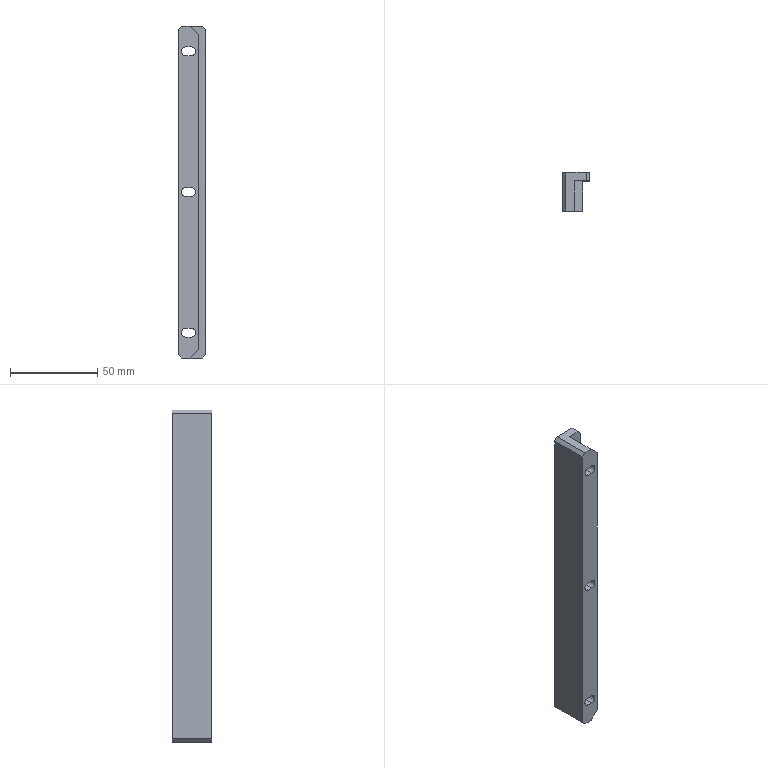Part | SolidWorks | features Chamfer 2, Extrusion 1, ICE 1 | 1 solid | 29 faces | box 16 x 22.5 x 190 mm | volume 52215 mm3 | plane 20 | cylinder 9 | commonest cylinder face diameters 5 x9
STEP:
#1=CARTESIAN_POINT('',(7.5,22.5,83.));
#2=VERTEX_POINT('',#1);
#3=CARTESIAN_POINT('',(10.,22.5,80.5));
#4=VERTEX_POINT('',#3);
#5=CARTESIAN_POINT('',(7.5,22.5,80.5));
#6=DIRECTION('',(0.,1.,0.));
#7=DIRECTION('',(0.,0.,-1.));
#8=AXIS2_PLACEMENT_3D('',#5,#6,#7);
#9=CIRCLE('',#8,2.5);
#10=EDGE_CURVE('',#2,#4,#9,.T.);
#11=ORIENTED_EDGE('',*,*,#10,.T.);
#12=CARTESIAN_POINT('',(10.,0.,80.5));
#13=VERTEX_POINT('',#12);
#14=CARTESIAN_POINT('',(10.,22.501,80.5));
#15=DIRECTION('',(0.,-1.,0.));
#16=VECTOR('',#15,1000.);
#17=LINE('',#14,#16);
#18=EDGE_CURVE('',#4,#13,#17,.T.);
#19=ORIENTED_EDGE('',*,*,#18,.T.);
#20=CARTESIAN_POINT('',(7.5,0.,83.));
#21=VERTEX_POINT('',#20);
#22=CARTESIAN_POINT('',(7.5,0.,80.5));
#23=DIRECTION('',(0.,-1.,0.));
#24=DIRECTION('',(1.,0.,0.));
#25=AXIS2_PLACEMENT_3D('',#22,#23,#24);
#26=CIRCLE('',#25,2.5);
#27=EDGE_CURVE('',#13,#21,#26,.T.);
#28=ORIENTED_EDGE('',*,*,#27,.T.);
#29=CARTESIAN_POINT('',(7.5,22.501,83.));
#30=DIRECTION('',(0.,-1.,0.));
#31=VECTOR('',#30,1000.);
#32=LINE('',#29,#31);
#33=EDGE_CURVE('',#2,#21,#32,.T.);
#34=ORIENTED_EDGE('',*,*,#33,.F.);
#35=EDGE_LOOP('',(#11,#19,#28,#34));
#36=FACE_OUTER_BOUND('',#35,.T.);
#37=CARTESIAN_POINT('',(7.5,22.501,80.5));
#38=DIRECTION('',(0.,-1.,0.));
#39=DIRECTION('',(1.,0.,0.));
#40=AXIS2_PLACEMENT_3D('',#37,#38,#39);
#41=CYLINDRICAL_SURFACE('',#40,2.5);
#42=ADVANCED_FACE('',(#36),#41,.F.);
#43=CARTESIAN_POINT('',(7.5,22.5,2.5));
#44=VERTEX_POINT('',#43);
#45=CARTESIAN_POINT('',(10.,22.5,0.));
#46=VERTEX_POINT('',#45);
#47=CARTESIAN_POINT('',(7.5,22.5,0.));
#48=DIRECTION('',(0.,1.,0.));
#49=DIRECTION('',(0.,0.,-1.));
#50=AXIS2_PLACEMENT_3D('',#47,#48,#49);
#51=CIRCLE('',#50,2.5);
#52=EDGE_CURVE('',#44,#46,#51,.T.);
#53=ORIENTED_EDGE('',*,*,#52,.T.);
#54=CARTESIAN_POINT('',(10.,0.,0.));
#55=VERTEX_POINT('',#54);
#56=CARTESIAN_POINT('',(10.,22.501,0.));
#57=DIRECTION('',(0.,-1.,0.));
#58=VECTOR('',#57,1000.);
#59=LINE('',#56,#58);
#60=EDGE_CURVE('',#46,#55,#59,.T.);
#61=ORIENTED_EDGE('',*,*,#60,.T.);
#62=CARTESIAN_POINT('',(7.5,0.,2.5));
#63=VERTEX_POINT('',#62);
#64=CARTESIAN_POINT('',(7.5,0.,0.));
#65=DIRECTION('',(0.,-1.,0.));
#66=DIRECTION('',(1.,0.,0.));
#67=AXIS2_PLACEMENT_3D('',#64,#65,#66);
#68=CIRCLE('',#67,2.5);
#69=EDGE_CURVE('',#55,#63,#68,.T.);
#70=ORIENTED_EDGE('',*,*,#69,.T.);
#71=CARTESIAN_POINT('',(7.5,22.501,2.5));
#72=DIRECTION('',(0.,-1.,0.));
#73=VECTOR('',#72,1000.);
#74=LINE('',#71,#73);
#75=EDGE_CURVE('',#44,#63,#74,.T.);
#76=ORIENTED_EDGE('',*,*,#75,.F.);
#77=EDGE_LOOP('',(#53,#61,#70,#76));
#78=FACE_OUTER_BOUND('',#77,.T.);
#79=CARTESIAN_POINT('',(7.5,22.501,0.));
#80=DIRECTION('',(0.,-1.,0.));
#81=DIRECTION('',(1.,0.,0.));
#82=AXIS2_PLACEMENT_3D('',#79,#80,#81);
#83=CYLINDRICAL_SURFACE('',#82,2.5);
#84=ADVANCED_FACE('',(#78),#83,.F.);
#85=CARTESIAN_POINT('',(7.5,22.5,-78.));
#86=VERTEX_POINT('',#85);
#87=CARTESIAN_POINT('',(10.,22.5,-80.5));
#88=VERTEX_POINT('',#87);
#89=CARTESIAN_POINT('',(7.5,22.5,-80.5));
#90=DIRECTION('',(0.,1.,0.));
#91=DIRECTION('',(0.,0.,-1.));
#92=AXIS2_PLACEMENT_3D('',#89,#90,#91);
#93=CIRCLE('',#92,2.5);
#94=EDGE_CURVE('',#86,#88,#93,.T.);
#95=ORIENTED_EDGE('',*,*,#94,.T.);
#96=CARTESIAN_POINT('',(10.,0.,-80.5));
#97=VERTEX_POINT('',#96);
#98=CARTESIAN_POINT('',(10.,22.501,-80.5));
#99=DIRECTION('',(0.,-1.,0.));
#100=VECTOR('',#99,1000.);
#101=LINE('',#98,#100);
#102=EDGE_CURVE('',#88,#97,#101,.T.);
#103=ORIENTED_EDGE('',*,*,#102,.T.);
#104=CARTESIAN_POINT('',(7.5,0.,-78.));
#105=VERTEX_POINT('',#104);
#106=CARTESIAN_POINT('',(7.5,0.,-80.5));
#107=DIRECTION('',(0.,-1.,0.));
#108=DIRECTION('',(-1.,0.,0.));
#109=AXIS2_PLACEMENT_3D('',#106,#107,#108);
#110=CIRCLE('',#109,2.5);
#111=EDGE_CURVE('',#97,#105,#110,.T.);
#112=ORIENTED_EDGE('',*,*,#111,.T.);
#113=CARTESIAN_POINT('',(7.5,22.501,-78.));
#114=DIRECTION('',(0.,-1.,0.));
#115=VECTOR('',#114,1000.);
#116=LINE('',#113,#115);
#117=EDGE_CURVE('',#86,#105,#116,.T.);
#118=ORIENTED_EDGE('',*,*,#117,.F.);
#119=EDGE_LOOP('',(#95,#103,#112,#118));
#120=FACE_OUTER_BOUND('',#119,.T.);
#121=CARTESIAN_POINT('',(7.5,22.501,-80.5));
#122=DIRECTION('',(0.,-1.,0.));
#123=DIRECTION('',(1.,0.,0.));
#124=AXIS2_PLACEMENT_3D('',#121,#122,#123);
#125=CYLINDRICAL_SURFACE('',#124,2.5);
#126=ADVANCED_FACE('',(#120),#125,.F.);
#127=CARTESIAN_POINT('',(4.5,0.,78.));
#128=VERTEX_POINT('',#127);
#129=CARTESIAN_POINT('',(7.5,0.,78.));
#130=VERTEX_POINT('',#129);
#131=CARTESIAN_POINT('',(4.5,0.,78.));
#132=DIRECTION('',(1.,0.,0.));
#133=VECTOR('',#132,1000.);
#134=LINE('',#131,#133);
#135=EDGE_CURVE('',#128,#130,#134,.T.);
#136=ORIENTED_EDGE('',*,*,#135,.F.);
#137=CARTESIAN_POINT('',(4.5,0.,83.));
#138=VERTEX_POINT('',#137);
#139=CARTESIAN_POINT('',(4.5,0.,80.5));
#140=DIRECTION('',(0.,-1.,0.));
#141=DIRECTION('',(1.,0.,0.));
#142=AXIS2_PLACEMENT_3D('',#139,#140,#141);
#143=CIRCLE('',#142,2.5);
#144=EDGE_CURVE('',#138,#128,#143,.T.);
#145=ORIENTED_EDGE('',*,*,#144,.F.);
#146=CARTESIAN_POINT('',(4.5,0.,83.));
#147=DIRECTION('',(-1.,0.,0.));
#148=VECTOR('',#147,1000.);
#149=LINE('',#146,#148);
#150=EDGE_CURVE('',#21,#138,#149,.T.);
#151=ORIENTED_EDGE('',*,*,#150,.F.);
#152=ORIENTED_EDGE('',*,*,#27,.F.);
#153=CARTESIAN_POINT('',(7.5,0.,80.5));
#154=DIRECTION('',(0.,-1.,0.));
#155=DIRECTION('',(1.,0.,0.));
#156=AXIS2_PLACEMENT_3D('',#153,#154,#155);
#157=CIRCLE('',#156,2.5);
#158=EDGE_CURVE('',#130,#13,#157,.T.);
#159=ORIENTED_EDGE('',*,*,#158,.F.);
#160=EDGE_LOOP('',(#136,#145,#151,#152,#159));
#161=FACE_BOUND('',#160,.T.);
#162=CARTESIAN_POINT('',(4.5,0.,-2.5));
#163=VERTEX_POINT('',#162);
#164=CARTESIAN_POINT('',(7.5,0.,-2.5));
#165=VERTEX_POINT('',#164);
#166=CARTESIAN_POINT('',(4.5,0.,-2.5));
#167=DIRECTION('',(1.,0.,0.));
#168=VECTOR('',#167,1000.);
#169=LINE('',#166,#168);
#170=EDGE_CURVE('',#163,#165,#169,.T.);
#171=ORIENTED_EDGE('',*,*,#170,.F.);
#172=CARTESIAN_POINT('',(4.5,0.,2.5));
#173=VERTEX_POINT('',#172);
#174=CARTESIAN_POINT('',(4.5,0.,0.));
#175=DIRECTION('',(0.,-1.,0.));
#176=DIRECTION('',(1.,0.,0.));
#177=AXIS2_PLACEMENT_3D('',#174,#175,#176);
#178=CIRCLE('',#177,2.5);
#179=EDGE_CURVE('',#173,#163,#178,.T.);
#180=ORIENTED_EDGE('',*,*,#179,.F.);
#181=CARTESIAN_POINT('',(4.5,0.,2.5));
#182=DIRECTION('',(-1.,0.,0.));
#183=VECTOR('',#182,1000.);
#184=LINE('',#181,#183);
#185=EDGE_CURVE('',#63,#173,#184,.T.);
#186=ORIENTED_EDGE('',*,*,#185,.F.);
#187=ORIENTED_EDGE('',*,*,#69,.F.);
#188=CARTESIAN_POINT('',(7.5,0.,0.));
#189=DIRECTION('',(0.,-1.,0.));
#190=DIRECTION('',(1.,0.,0.));
#191=AXIS2_PLACEMENT_3D('',#188,#189,#190);
#192=CIRCLE('',#191,2.5);
#193=EDGE_CURVE('',#165,#55,#192,.T.);
#194=ORIENTED_EDGE('',*,*,#193,.F.);
#195=EDGE_LOOP('',(#171,#180,#186,#187,#194));
#196=FACE_BOUND('',#195,.T.);
#197=CARTESIAN_POINT('',(4.5,0.,-83.));
#198=VERTEX_POINT('',#197);
#199=CARTESIAN_POINT('',(7.5,0.,-83.));
#200=VERTEX_POINT('',#199);
#201=CARTESIAN_POINT('',(4.5,0.,-83.));
#202=DIRECTION('',(1.,0.,0.));
#203=VECTOR('',#202,1000.);
#204=LINE('',#201,#203);
#205=EDGE_CURVE('',#198,#200,#204,.T.);
#206=ORIENTED_EDGE('',*,*,#205,.F.);
#207=CARTESIAN_POINT('',(4.5,0.,-78.));
#208=VERTEX_POINT('',#207);
#209=CARTESIAN_POINT('',(4.5,0.,-80.5));
#210=DIRECTION('',(0.,-1.,0.));
#211=DIRECTION('',(-1.,0.,0.));
#212=AXIS2_PLACEMENT_3D('',#209,#210,#211);
#213=CIRCLE('',#212,2.5);
#214=EDGE_CURVE('',#208,#198,#213,.T.);
#215=ORIENTED_EDGE('',*,*,#214,.F.);
#216=CARTESIAN_POINT('',(4.5,0.,-78.));
#217=DIRECTION('',(-1.,0.,0.));
#218=VECTOR('',#217,1000.);
#219=LINE('',#216,#218);
#220=EDGE_CURVE('',#105,#208,#219,.T.);
#221=ORIENTED_EDGE('',*,*,#220,.F.);
#222=ORIENTED_EDGE('',*,*,#111,.F.);
#223=CARTESIAN_POINT('',(7.5,0.,-80.5));
#224=DIRECTION('',(0.,-1.,0.));
#225=DIRECTION('',(-1.,0.,0.));
#226=AXIS2_PLACEMENT_3D('',#223,#224,#225);
#227=CIRCLE('',#226,2.5);
#228=EDGE_CURVE('',#200,#97,#227,.T.);
#229=ORIENTED_EDGE('',*,*,#228,.F.);
#230=EDGE_LOOP('',(#206,#215,#221,#222,#229));
#231=FACE_BOUND('',#230,.T.);
#232=CARTESIAN_POINT('',(2.,0.,95.));
#233=VERTEX_POINT('',#232);
#234=CARTESIAN_POINT('',(7.,0.,95.));
#235=VERTEX_POINT('',#234);
#236=CARTESIAN_POINT('',(12.,0.,95.));
#237=DIRECTION('',(1.,0.,0.));
#238=VECTOR('',#237,1000.);
#239=LINE('',#236,#238);
#240=EDGE_CURVE('',#233,#235,#239,.T.);
#241=ORIENTED_EDGE('',*,*,#240,.F.);
#242=CARTESIAN_POINT('',(0.,0.,93.));
#243=VERTEX_POINT('',#242);
#244=CARTESIAN_POINT('',(2.,0.,95.));
#245=DIRECTION('',(-0.7071,0.,-0.7071));
#246=VECTOR('',#245,1000.);
#247=LINE('',#244,#246);
#248=EDGE_CURVE('',#233,#243,#247,.T.);
#249=ORIENTED_EDGE('',*,*,#248,.T.);
#250=CARTESIAN_POINT('',(0.,0.,-93.));
#251=VERTEX_POINT('',#250);
#252=CARTESIAN_POINT('',(0.,0.,95.));
#253=DIRECTION('',(0.,0.,-1.));
#254=VECTOR('',#253,1000.);
#255=LINE('',#252,#254);
#256=EDGE_CURVE('',#243,#251,#255,.T.);
#257=ORIENTED_EDGE('',*,*,#256,.T.);
#258=CARTESIAN_POINT('',(2.,0.,-95.));
#259=VERTEX_POINT('',#258);
#260=CARTESIAN_POINT('',(0.,0.,-93.));
#261=DIRECTION('',(0.7071,0.,-0.7071));
#262=VECTOR('',#261,1000.);
#263=LINE('',#260,#262);
#264=EDGE_CURVE('',#251,#259,#263,.T.);
#265=ORIENTED_EDGE('',*,*,#264,.T.);
#266=CARTESIAN_POINT('',(7.,0.,-95.));
#267=VERTEX_POINT('',#266);
#268=CARTESIAN_POINT('',(12.,0.,-95.));
#269=DIRECTION('',(1.,0.,0.));
#270=VECTOR('',#269,1000.);
#271=LINE('',#268,#270);
#272=EDGE_CURVE('',#259,#267,#271,.T.);
#273=ORIENTED_EDGE('',*,*,#272,.T.);
#274=CARTESIAN_POINT('',(12.,0.,-90.));
#275=VERTEX_POINT('',#274);
#276=CARTESIAN_POINT('',(12.,0.,-90.));
#277=DIRECTION('',(0.7071,0.,0.7071));
#278=VECTOR('',#277,1000.);
#279=LINE('',#276,#278);
#280=EDGE_CURVE('',#267,#275,#279,.T.);
#281=ORIENTED_EDGE('',*,*,#280,.T.);
#282=CARTESIAN_POINT('',(12.,0.,90.));
#283=VERTEX_POINT('',#282);
#284=CARTESIAN_POINT('',(12.,0.,95.));
#285=DIRECTION('',(0.,0.,-1.));
#286=VECTOR('',#285,1000.);
#287=LINE('',#284,#286);
#288=EDGE_CURVE('',#283,#275,#287,.T.);
#289=ORIENTED_EDGE('',*,*,#288,.F.);
#290=CARTESIAN_POINT('',(7.,0.,95.));
#291=DIRECTION('',(-0.7071,0.,0.7071));
#292=VECTOR('',#291,1000.);
#293=LINE('',#290,#292);
#294=EDGE_CURVE('',#283,#235,#293,.T.);
#295=ORIENTED_EDGE('',*,*,#294,.T.);
#296=EDGE_LOOP('',(#241,#249,#257,#265,#273,#281,#289,#295));
#297=FACE_OUTER_BOUND('',#296,.T.);
#298=CARTESIAN_POINT('',(12.,0.,95.));
#299=DIRECTION('',(0.,1.,0.));
#300=DIRECTION('',(-1.,0.,0.));
#301=AXIS2_PLACEMENT_3D('',#298,#299,#300);
#302=PLANE('',#301);
#303=ADVANCED_FACE('',(#161,#196,#231,#297),#302,.F.);
#304=ORIENTED_EDGE('',*,*,#288,.T.);
#305=CARTESIAN_POINT('',(12.,17.5,-90.));
#306=VERTEX_POINT('',#305);
#307=CARTESIAN_POINT('',(12.,17.5,-90.));
#308=DIRECTION('',(0.,1.,0.));
#309=VECTOR('',#308,1000.);
#310=LINE('',#307,#309);
#311=EDGE_CURVE('',#275,#306,#310,.T.);
#312=ORIENTED_EDGE('',*,*,#311,.T.);
#313=CARTESIAN_POINT('',(12.,17.5,90.));
#314=VERTEX_POINT('',#313);
#315=CARTESIAN_POINT('',(12.,17.5,95.));
#316=DIRECTION('',(0.,0.,-1.));
#317=VECTOR('',#316,1000.);
#318=LINE('',#315,#317);
#319=EDGE_CURVE('',#314,#306,#318,.T.);
#320=ORIENTED_EDGE('',*,*,#319,.F.);
#321=CARTESIAN_POINT('',(12.,17.5,90.));
#322=DIRECTION('',(0.,-1.,0.));
#323=VECTOR('',#322,1000.);
#324=LINE('',#321,#323);
#325=EDGE_CURVE('',#314,#283,#324,.T.);
#326=ORIENTED_EDGE('',*,*,#325,.T.);
#327=EDGE_LOOP('',(#304,#312,#320,#326));
#328=FACE_OUTER_BOUND('',#327,.T.);
#329=CARTESIAN_POINT('',(12.,17.5,95.));
#330=DIRECTION('',(-1.,0.,0.));
#331=DIRECTION('',(0.,-1.,0.));
#332=AXIS2_PLACEMENT_3D('',#329,#330,#331);
#333=PLANE('',#332);
#334=ADVANCED_FACE('',(#328),#333,.F.);
#335=CARTESIAN_POINT('',(7.,17.5,-95.));
#336=VERTEX_POINT('',#335);
#337=CARTESIAN_POINT('',(14.,17.5,-95.));
#338=VERTEX_POINT('',#337);
#339=CARTESIAN_POINT('',(16.,17.5,-95.));
#340=DIRECTION('',(1.,0.,0.));
#341=VECTOR('',#340,1000.);
#342=LINE('',#339,#341);
#343=EDGE_CURVE('',#336,#338,#342,.T.);
#344=ORIENTED_EDGE('',*,*,#343,.T.);
#345=CARTESIAN_POINT('',(16.,17.5,-93.));
#346=VERTEX_POINT('',#345);
#347=CARTESIAN_POINT('',(16.,17.5,-93.));
#348=DIRECTION('',(0.7071,0.,0.7071));
#349=VECTOR('',#348,1000.);
#350=LINE('',#347,#349);
#351=EDGE_CURVE('',#338,#346,#350,.T.);
#352=ORIENTED_EDGE('',*,*,#351,.T.);
#353=CARTESIAN_POINT('',(16.,17.5,93.));
#354=VERTEX_POINT('',#353);
#355=CARTESIAN_POINT('',(16.,17.5,95.));
#356=DIRECTION('',(0.,0.,-1.));
#357=VECTOR('',#356,1000.);
#358=LINE('',#355,#357);
#359=EDGE_CURVE('',#354,#346,#358,.T.);
#360=ORIENTED_EDGE('',*,*,#359,.F.);
#361=CARTESIAN_POINT('',(14.,17.5,95.));
#362=VERTEX_POINT('',#361);
#363=CARTESIAN_POINT('',(14.,17.5,95.));
#364=DIRECTION('',(-0.7071,0.,0.7071));
#365=VECTOR('',#364,1000.);
#366=LINE('',#363,#365);
#367=EDGE_CURVE('',#354,#362,#366,.T.);
#368=ORIENTED_EDGE('',*,*,#367,.T.);
#369=CARTESIAN_POINT('',(7.,17.5,95.));
#370=VERTEX_POINT('',#369);
#371=CARTESIAN_POINT('',(16.,17.5,95.));
#372=DIRECTION('',(1.,0.,0.));
#373=VECTOR('',#372,1000.);
#374=LINE('',#371,#373);
#375=EDGE_CURVE('',#370,#362,#374,.T.);
#376=ORIENTED_EDGE('',*,*,#375,.F.);
#377=CARTESIAN_POINT('',(11.5,17.5,90.5));
#378=DIRECTION('',(0.7071,0.,-0.7071));
#379=VECTOR('',#378,1000.);
#380=LINE('',#377,#379);
#381=EDGE_CURVE('',#370,#314,#380,.T.);
#382=ORIENTED_EDGE('',*,*,#381,.T.);
#383=ORIENTED_EDGE('',*,*,#319,.T.);
#384=CARTESIAN_POINT('',(106.5,17.5,4.5));
#385=DIRECTION('',(-0.7071,0.,-0.7071));
#386=VECTOR('',#385,1000.);
#387=LINE('',#384,#386);
#388=EDGE_CURVE('',#306,#336,#387,.T.);
#389=ORIENTED_EDGE('',*,*,#388,.T.);
#390=EDGE_LOOP('',(#344,#352,#360,#368,#376,#382,#383,#389));
#391=FACE_OUTER_BOUND('',#390,.T.);
#392=CARTESIAN_POINT('',(16.,17.5,95.));
#393=DIRECTION('',(0.,1.,0.));
#394=DIRECTION('',(0.,0.,1.));
#395=AXIS2_PLACEMENT_3D('',#392,#393,#394);
#396=PLANE('',#395);
#397=ADVANCED_FACE('',(#391),#396,.F.);
#398=ORIENTED_EDGE('',*,*,#359,.T.);
#399=CARTESIAN_POINT('',(16.,22.5,-93.));
#400=VERTEX_POINT('',#399);
#401=CARTESIAN_POINT('',(16.,22.5,-93.));
#402=DIRECTION('',(0.,1.,0.));
#403=VECTOR('',#402,1000.);
#404=LINE('',#401,#403);
#405=EDGE_CURVE('',#346,#400,#404,.T.);
#406=ORIENTED_EDGE('',*,*,#405,.T.);
#407=CARTESIAN_POINT('',(16.,22.5,93.));
#408=VERTEX_POINT('',#407);
#409=CARTESIAN_POINT('',(16.,22.5,95.));
#410=DIRECTION('',(0.,0.,-1.));
#411=VECTOR('',#410,1000.);
#412=LINE('',#409,#411);
#413=EDGE_CURVE('',#408,#400,#412,.T.);
#414=ORIENTED_EDGE('',*,*,#413,.F.);
#415=CARTESIAN_POINT('',(16.,22.5,93.));
#416=DIRECTION('',(0.,-1.,0.));
#417=VECTOR('',#416,1000.);
#418=LINE('',#415,#417);
#419=EDGE_CURVE('',#408,#354,#418,.T.);
#420=ORIENTED_EDGE('',*,*,#419,.T.);
#421=EDGE_LOOP('',(#398,#406,#414,#420));
#422=FACE_OUTER_BOUND('',#421,.T.);
#423=CARTESIAN_POINT('',(16.,22.5,95.));
#424=DIRECTION('',(-1.,0.,0.));
#425=DIRECTION('',(0.,0.,1.));
#426=AXIS2_PLACEMENT_3D('',#423,#424,#425);
#427=PLANE('',#426);
#428=ADVANCED_FACE('',(#422),#427,.F.);
#429=CARTESIAN_POINT('',(4.5,22.5,83.));
#430=VERTEX_POINT('',#429);
#431=CARTESIAN_POINT('',(4.5,22.5,83.));
#432=DIRECTION('',(1.,0.,0.));
#433=VECTOR('',#432,1000.);
#434=LINE('',#431,#433);
#435=EDGE_CURVE('',#430,#2,#434,.T.);
#436=ORIENTED_EDGE('',*,*,#435,.F.);
#437=CARTESIAN_POINT('',(4.5,22.5,78.));
#438=VERTEX_POINT('',#437);
#439=CARTESIAN_POINT('',(4.5,22.5,80.5));
#440=DIRECTION('',(0.,1.,0.));
#441=DIRECTION('',(0.,0.,-1.));
#442=AXIS2_PLACEMENT_3D('',#439,#440,#441);
#443=CIRCLE('',#442,2.5);
#444=EDGE_CURVE('',#438,#430,#443,.T.);
#445=ORIENTED_EDGE('',*,*,#444,.F.);
#446=CARTESIAN_POINT('',(7.5,22.5,78.));
#447=VERTEX_POINT('',#446);
#448=CARTESIAN_POINT('',(4.5,22.5,78.));
#449=DIRECTION('',(-1.,0.,0.));
#450=VECTOR('',#449,1000.);
#451=LINE('',#448,#450);
#452=EDGE_CURVE('',#447,#438,#451,.T.);
#453=ORIENTED_EDGE('',*,*,#452,.F.);
#454=CARTESIAN_POINT('',(7.5,22.5,80.5));
#455=DIRECTION('',(0.,1.,0.));
#456=DIRECTION('',(0.,0.,-1.));
#457=AXIS2_PLACEMENT_3D('',#454,#455,#456);
#458=CIRCLE('',#457,2.5);
#459=EDGE_CURVE('',#4,#447,#458,.T.);
#460=ORIENTED_EDGE('',*,*,#459,.F.);
#461=ORIENTED_EDGE('',*,*,#10,.F.);
#462=EDGE_LOOP('',(#436,#445,#453,#460,#461));
#463=FACE_BOUND('',#462,.T.);
#464=CARTESIAN_POINT('',(4.5,22.5,2.5));
#465=VERTEX_POINT('',#464);
#466=CARTESIAN_POINT('',(4.5,22.5,2.5));
#467=DIRECTION('',(1.,0.,0.));
#468=VECTOR('',#467,1000.);
#469=LINE('',#466,#468);
#470=EDGE_CURVE('',#465,#44,#469,.T.);
#471=ORIENTED_EDGE('',*,*,#470,.F.);
#472=CARTESIAN_POINT('',(4.5,22.5,-2.5));
#473=VERTEX_POINT('',#472);
#474=CARTESIAN_POINT('',(4.5,22.5,0.));
#475=DIRECTION('',(0.,1.,0.));
#476=DIRECTION('',(0.,0.,-1.));
#477=AXIS2_PLACEMENT_3D('',#474,#475,#476);
#478=CIRCLE('',#477,2.5);
#479=EDGE_CURVE('',#473,#465,#478,.T.);
#480=ORIENTED_EDGE('',*,*,#479,.F.);
#481=CARTESIAN_POINT('',(7.5,22.5,-2.5));
#482=VERTEX_POINT('',#481);
#483=CARTESIAN_POINT('',(4.5,22.5,-2.5));
#484=DIRECTION('',(-1.,0.,0.));
#485=VECTOR('',#484,1000.);
#486=LINE('',#483,#485);
#487=EDGE_CURVE('',#482,#473,#486,.T.);
#488=ORIENTED_EDGE('',*,*,#487,.F.);
#489=CARTESIAN_POINT('',(7.5,22.5,0.));
#490=DIRECTION('',(0.,1.,0.));
#491=DIRECTION('',(0.,0.,-1.));
#492=AXIS2_PLACEMENT_3D('',#489,#490,#491);
#493=CIRCLE('',#492,2.5);
#494=EDGE_CURVE('',#46,#482,#493,.T.);
#495=ORIENTED_EDGE('',*,*,#494,.F.);
#496=ORIENTED_EDGE('',*,*,#52,.F.);
#497=EDGE_LOOP('',(#471,#480,#488,#495,#496));
#498=FACE_BOUND('',#497,.T.);
#499=CARTESIAN_POINT('',(4.5,22.5,-78.));
#500=VERTEX_POINT('',#499);
#501=CARTESIAN_POINT('',(4.5,22.5,-78.));
#502=DIRECTION('',(1.,0.,0.));
#503=VECTOR('',#502,1000.);
#504=LINE('',#501,#503);
#505=EDGE_CURVE('',#500,#86,#504,.T.);
#506=ORIENTED_EDGE('',*,*,#505,.F.);
#507=CARTESIAN_POINT('',(4.5,22.5,-83.));
#508=VERTEX_POINT('',#507);
#509=CARTESIAN_POINT('',(4.5,22.5,-80.5));
#510=DIRECTION('',(0.,1.,0.));
#511=DIRECTION('',(0.,0.,-1.));
#512=AXIS2_PLACEMENT_3D('',#509,#510,#511);
#513=CIRCLE('',#512,2.5);
#514=EDGE_CURVE('',#508,#500,#513,.T.);
#515=ORIENTED_EDGE('',*,*,#514,.F.);
#516=CARTESIAN_POINT('',(7.5,22.5,-83.));
#517=VERTEX_POINT('',#516);
#518=CARTESIAN_POINT('',(4.5,22.5,-83.));
#519=DIRECTION('',(-1.,0.,0.));
#520=VECTOR('',#519,1000.);
#521=LINE('',#518,#520);
#522=EDGE_CURVE('',#517,#508,#521,.T.);
#523=ORIENTED_EDGE('',*,*,#522,.F.);
#524=CARTESIAN_POINT('',(7.5,22.5,-80.5));
#525=DIRECTION('',(0.,1.,0.));
#526=DIRECTION('',(0.,0.,-1.));
#527=AXIS2_PLACEMENT_3D('',#524,#525,#526);
#528=CIRCLE('',#527,2.5);
#529=EDGE_CURVE('',#88,#517,#528,.T.);
#530=ORIENTED_EDGE('',*,*,#529,.F.);
#531=ORIENTED_EDGE('',*,*,#94,.F.);
#532=EDGE_LOOP('',(#506,#515,#523,#530,#531));
#533=FACE_BOUND('',#532,.T.);
#534=CARTESIAN_POINT('',(0.,22.5,93.));
#535=VERTEX_POINT('',#534);
#536=CARTESIAN_POINT('',(0.,22.5,-93.));
#537=VERTEX_POINT('',#536);
#538=CARTESIAN_POINT('',(0.,22.5,95.));
#539=DIRECTION('',(0.,0.,-1.));
#540=VECTOR('',#539,1000.);
#541=LINE('',#538,#540);
#542=EDGE_CURVE('',#535,#537,#541,.T.);
#543=ORIENTED_EDGE('',*,*,#542,.F.);
#544=CARTESIAN_POINT('',(2.,22.5,95.));
#545=VERTEX_POINT('',#544);
#546=CARTESIAN_POINT('',(2.,22.5,95.));
#547=DIRECTION('',(0.7071,0.,0.7071));
#548=VECTOR('',#547,1000.);
#549=LINE('',#546,#548);
#550=EDGE_CURVE('',#535,#545,#549,.T.);
#551=ORIENTED_EDGE('',*,*,#550,.T.);
#552=CARTESIAN_POINT('',(14.,22.5,95.));
#553=VERTEX_POINT('',#552);
#554=CARTESIAN_POINT('',(0.,22.5,95.));
#555=DIRECTION('',(-1.,0.,0.));
#556=VECTOR('',#555,1000.);
#557=LINE('',#554,#556);
#558=EDGE_CURVE('',#553,#545,#557,.T.);
#559=ORIENTED_EDGE('',*,*,#558,.F.);
#560=CARTESIAN_POINT('',(14.,22.5,95.));
#561=DIRECTION('',(0.7071,0.,-0.7071));
#562=VECTOR('',#561,1000.);
#563=LINE('',#560,#562);
#564=EDGE_CURVE('',#553,#408,#563,.T.);
#565=ORIENTED_EDGE('',*,*,#564,.T.);
#566=ORIENTED_EDGE('',*,*,#413,.T.);
#567=CARTESIAN_POINT('',(14.,22.5,-95.));
#568=VERTEX_POINT('',#567);
#569=CARTESIAN_POINT('',(16.,22.5,-93.));
#570=DIRECTION('',(-0.7071,0.,-0.7071));
#571=VECTOR('',#570,1000.);
#572=LINE('',#569,#571);
#573=EDGE_CURVE('',#400,#568,#572,.T.);
#574=ORIENTED_EDGE('',*,*,#573,.T.);
#575=CARTESIAN_POINT('',(2.,22.5,-95.));
#576=VERTEX_POINT('',#575);
#577=CARTESIAN_POINT('',(0.,22.5,-95.));
#578=DIRECTION('',(-1.,0.,0.));
#579=VECTOR('',#578,1000.);
#580=LINE('',#577,#579);
#581=EDGE_CURVE('',#568,#576,#580,.T.);
#582=ORIENTED_EDGE('',*,*,#581,.T.);
#583=CARTESIAN_POINT('',(0.,22.5,-93.));
#584=DIRECTION('',(-0.7071,0.,0.7071));
#585=VECTOR('',#584,1000.);
#586=LINE('',#583,#585);
#587=EDGE_CURVE('',#576,#537,#586,.T.);
#588=ORIENTED_EDGE('',*,*,#587,.T.);
#589=EDGE_LOOP('',(#543,#551,#559,#565,#566,#574,#582,#588));
#590=FACE_OUTER_BOUND('',#589,.T.);
#591=CARTESIAN_POINT('',(0.,22.5,95.));
#592=DIRECTION('',(0.,-1.,0.));
#593=DIRECTION('',(0.,0.,-1.));
#594=AXIS2_PLACEMENT_3D('',#591,#592,#593);
#595=PLANE('',#594);
#596=ADVANCED_FACE('',(#463,#498,#533,#590),#595,.F.);
#597=ORIENTED_EDGE('',*,*,#256,.F.);
#598=CARTESIAN_POINT('',(0.,0.,93.));
#599=DIRECTION('',(0.,1.,0.));
#600=VECTOR('',#599,1000.);
#601=LINE('',#598,#600);
#602=EDGE_CURVE('',#243,#535,#601,.T.);
#603=ORIENTED_EDGE('',*,*,#602,.T.);
#604=ORIENTED_EDGE('',*,*,#542,.T.);
#605=CARTESIAN_POINT('',(0.,0.,-93.));
#606=DIRECTION('',(0.,-1.,0.));
#607=VECTOR('',#606,1000.);
#608=LINE('',#605,#607);
#609=EDGE_CURVE('',#537,#251,#608,.T.);
#610=ORIENTED_EDGE('',*,*,#609,.T.);
#611=EDGE_LOOP('',(#597,#603,#604,#610));
#612=FACE_OUTER_BOUND('',#611,.T.);
#613=CARTESIAN_POINT('',(0.,0.,95.));
#614=DIRECTION('',(1.,0.,0.));
#615=DIRECTION('',(0.,0.,-1.));
#616=AXIS2_PLACEMENT_3D('',#613,#614,#615);
#617=PLANE('',#616);
#618=ADVANCED_FACE('',(#612),#617,.F.);
#619=ORIENTED_EDGE('',*,*,#558,.T.);
#620=CARTESIAN_POINT('',(2.,0.,95.));
#621=DIRECTION('',(0.,-1.,0.));
#622=VECTOR('',#621,1000.);
#623=LINE('',#620,#622);
#624=EDGE_CURVE('',#545,#233,#623,.T.);
#625=ORIENTED_EDGE('',*,*,#624,.T.);
#626=ORIENTED_EDGE('',*,*,#240,.T.);
#627=CARTESIAN_POINT('',(7.,0.,95.));
#628=DIRECTION('',(0.,1.,0.));
#629=VECTOR('',#628,1000.);
#630=LINE('',#627,#629);
#631=EDGE_CURVE('',#235,#370,#630,.T.);
#632=ORIENTED_EDGE('',*,*,#631,.T.);
#633=ORIENTED_EDGE('',*,*,#375,.T.);
#634=CARTESIAN_POINT('',(14.,0.,95.));
#635=DIRECTION('',(0.,1.,0.));
#636=VECTOR('',#635,1000.);
#637=LINE('',#634,#636);
#638=EDGE_CURVE('',#362,#553,#637,.T.);
#639=ORIENTED_EDGE('',*,*,#638,.T.);
#640=EDGE_LOOP('',(#619,#625,#626,#632,#633,#639));
#641=FACE_OUTER_BOUND('',#640,.T.);
#642=CARTESIAN_POINT('',(0.,0.,95.));
#643=DIRECTION('',(0.,0.,-1.));
#644=DIRECTION('',(-1.,0.,0.));
#645=AXIS2_PLACEMENT_3D('',#642,#643,#644);
#646=PLANE('',#645);
#647=ADVANCED_FACE('',(#641),#646,.F.);
#648=ORIENTED_EDGE('',*,*,#272,.F.);
#649=CARTESIAN_POINT('',(2.,22.5,-95.));
#650=DIRECTION('',(0.,1.,0.));
#651=VECTOR('',#650,1000.);
#652=LINE('',#649,#651);
#653=EDGE_CURVE('',#259,#576,#652,.T.);
#654=ORIENTED_EDGE('',*,*,#653,.T.);
#655=ORIENTED_EDGE('',*,*,#581,.F.);
#656=CARTESIAN_POINT('',(14.,17.5,-95.));
#657=DIRECTION('',(0.,-1.,0.));
#658=VECTOR('',#657,1000.);
#659=LINE('',#656,#658);
#660=EDGE_CURVE('',#568,#338,#659,.T.);
#661=ORIENTED_EDGE('',*,*,#660,.T.);
#662=ORIENTED_EDGE('',*,*,#343,.F.);
#663=CARTESIAN_POINT('',(7.,0.,-95.));
#664=DIRECTION('',(0.,-1.,0.));
#665=VECTOR('',#664,1000.);
#666=LINE('',#663,#665);
#667=EDGE_CURVE('',#336,#267,#666,.T.);
#668=ORIENTED_EDGE('',*,*,#667,.T.);
#669=EDGE_LOOP('',(#648,#654,#655,#661,#662,#668));
#670=FACE_OUTER_BOUND('',#669,.T.);
#671=CARTESIAN_POINT('',(0.,0.,-95.));
#672=DIRECTION('',(0.,0.,-1.));
#673=DIRECTION('',(-1.,0.,0.));
#674=AXIS2_PLACEMENT_3D('',#671,#672,#673);
#675=PLANE('',#674);
#676=ADVANCED_FACE('',(#670),#675,.T.);
#677=ORIENTED_EDGE('',*,*,#280,.F.);
#678=ORIENTED_EDGE('',*,*,#667,.F.);
#679=ORIENTED_EDGE('',*,*,#388,.F.);
#680=ORIENTED_EDGE('',*,*,#311,.F.);
#681=EDGE_LOOP('',(#677,#678,#679,#680));
#682=FACE_OUTER_BOUND('',#681,.T.);
#683=CARTESIAN_POINT('',(12.,17.5,-90.));
#684=DIRECTION('',(0.7071,0.,-0.7071));
#685=DIRECTION('',(0.,-1.,0.));
#686=AXIS2_PLACEMENT_3D('',#683,#684,#685);
#687=PLANE('',#686);
#688=ADVANCED_FACE('',(#682),#687,.T.);
#689=ORIENTED_EDGE('',*,*,#294,.F.);
#690=ORIENTED_EDGE('',*,*,#325,.F.);
#691=ORIENTED_EDGE('',*,*,#381,.F.);
#692=ORIENTED_EDGE('',*,*,#631,.F.);
#693=EDGE_LOOP('',(#689,#690,#691,#692));
#694=FACE_OUTER_BOUND('',#693,.T.);
#695=CARTESIAN_POINT('',(7.,0.,95.));
#696=DIRECTION('',(-0.7071,0.,-0.7071));
#697=DIRECTION('',(0.,1.,0.));
#698=AXIS2_PLACEMENT_3D('',#695,#696,#697);
#699=PLANE('',#698);
#700=ADVANCED_FACE('',(#694),#699,.F.);
#701=ORIENTED_EDGE('',*,*,#550,.F.);
#702=ORIENTED_EDGE('',*,*,#602,.F.);
#703=ORIENTED_EDGE('',*,*,#248,.F.);
#704=ORIENTED_EDGE('',*,*,#624,.F.);
#705=EDGE_LOOP('',(#701,#702,#703,#704));
#706=FACE_OUTER_BOUND('',#705,.T.);
#707=CARTESIAN_POINT('',(2.,0.,95.));
#708=DIRECTION('',(0.7071,0.,-0.7071));
#709=DIRECTION('',(0.,-1.,0.));
#710=AXIS2_PLACEMENT_3D('',#707,#708,#709);
#711=PLANE('',#710);
#712=ADVANCED_FACE('',(#706),#711,.F.);
#713=ORIENTED_EDGE('',*,*,#587,.F.);
#714=ORIENTED_EDGE('',*,*,#653,.F.);
#715=ORIENTED_EDGE('',*,*,#264,.F.);
#716=ORIENTED_EDGE('',*,*,#609,.F.);
#717=EDGE_LOOP('',(#713,#714,#715,#716));
#718=FACE_OUTER_BOUND('',#717,.T.);
#719=CARTESIAN_POINT('',(0.,0.,-93.));
#720=DIRECTION('',(-0.7071,0.,-0.7071));
#721=DIRECTION('',(0.,1.,0.));
#722=AXIS2_PLACEMENT_3D('',#719,#720,#721);
#723=PLANE('',#722);
#724=ADVANCED_FACE('',(#718),#723,.T.);
#725=ORIENTED_EDGE('',*,*,#351,.F.);
#726=ORIENTED_EDGE('',*,*,#660,.F.);
#727=ORIENTED_EDGE('',*,*,#573,.F.);
#728=ORIENTED_EDGE('',*,*,#405,.F.);
#729=EDGE_LOOP('',(#725,#726,#727,#728));
#730=FACE_OUTER_BOUND('',#729,.T.);
#731=CARTESIAN_POINT('',(16.,22.5,-93.));
#732=DIRECTION('',(0.7071,0.,-0.7071));
#733=DIRECTION('',(0.,-1.,0.));
#734=AXIS2_PLACEMENT_3D('',#731,#732,#733);
#735=PLANE('',#734);
#736=ADVANCED_FACE('',(#730),#735,.T.);
#737=ORIENTED_EDGE('',*,*,#367,.F.);
#738=ORIENTED_EDGE('',*,*,#419,.F.);
#739=ORIENTED_EDGE('',*,*,#564,.F.);
#740=ORIENTED_EDGE('',*,*,#638,.F.);
#741=EDGE_LOOP('',(#737,#738,#739,#740));
#742=FACE_OUTER_BOUND('',#741,.T.);
#743=CARTESIAN_POINT('',(14.,0.,95.));
#744=DIRECTION('',(-0.7071,0.,-0.7071));
#745=DIRECTION('',(0.,1.,0.));
#746=AXIS2_PLACEMENT_3D('',#743,#744,#745);
#747=PLANE('',#746);
#748=ADVANCED_FACE('',(#742),#747,.F.);
#749=ORIENTED_EDGE('',*,*,#514,.T.);
#750=CARTESIAN_POINT('',(4.5,22.501,-78.));
#751=DIRECTION('',(0.,-1.,0.));
#752=VECTOR('',#751,1000.);
#753=LINE('',#750,#752);
#754=EDGE_CURVE('',#500,#208,#753,.T.);
#755=ORIENTED_EDGE('',*,*,#754,.T.);
#756=ORIENTED_EDGE('',*,*,#214,.T.);
#757=CARTESIAN_POINT('',(4.5,22.501,-83.));
#758=DIRECTION('',(0.,-1.,0.));
#759=VECTOR('',#758,1000.);
#760=LINE('',#757,#759);
#761=EDGE_CURVE('',#508,#198,#760,.T.);
#762=ORIENTED_EDGE('',*,*,#761,.F.);
#763=EDGE_LOOP('',(#749,#755,#756,#762));
#764=FACE_OUTER_BOUND('',#763,.T.);
#765=CARTESIAN_POINT('',(4.5,22.501,-80.5));
#766=DIRECTION('',(0.,-1.,0.));
#767=DIRECTION('',(1.,0.,0.));
#768=AXIS2_PLACEMENT_3D('',#765,#766,#767);
#769=CYLINDRICAL_SURFACE('',#768,2.5);
#770=ADVANCED_FACE('',(#764),#769,.F.);
#771=ORIENTED_EDGE('',*,*,#505,.T.);
#772=ORIENTED_EDGE('',*,*,#117,.T.);
#773=ORIENTED_EDGE('',*,*,#220,.T.);
#774=ORIENTED_EDGE('',*,*,#754,.F.);
#775=EDGE_LOOP('',(#771,#772,#773,#774));
#776=FACE_OUTER_BOUND('',#775,.T.);
#777=CARTESIAN_POINT('',(4.5,22.501,-78.));
#778=DIRECTION('',(0.,0.,1.));
#779=DIRECTION('',(1.,0.,0.));
#780=AXIS2_PLACEMENT_3D('',#777,#778,#779);
#781=PLANE('',#780);
#782=ADVANCED_FACE('',(#776),#781,.F.);
#783=ORIENTED_EDGE('',*,*,#102,.F.);
#784=ORIENTED_EDGE('',*,*,#529,.T.);
#785=CARTESIAN_POINT('',(7.5,22.501,-83.));
#786=DIRECTION('',(0.,-1.,0.));
#787=VECTOR('',#786,1000.);
#788=LINE('',#785,#787);
#789=EDGE_CURVE('',#517,#200,#788,.T.);
#790=ORIENTED_EDGE('',*,*,#789,.T.);
#791=ORIENTED_EDGE('',*,*,#228,.T.);
#792=EDGE_LOOP('',(#783,#784,#790,#791));
#793=FACE_OUTER_BOUND('',#792,.T.);
#794=CARTESIAN_POINT('',(7.5,22.501,-80.5));
#795=DIRECTION('',(0.,-1.,0.));
#796=DIRECTION('',(1.,0.,0.));
#797=AXIS2_PLACEMENT_3D('',#794,#795,#796);
#798=CYLINDRICAL_SURFACE('',#797,2.5);
#799=ADVANCED_FACE('',(#793),#798,.F.);
#800=ORIENTED_EDGE('',*,*,#522,.T.);
#801=ORIENTED_EDGE('',*,*,#761,.T.);
#802=ORIENTED_EDGE('',*,*,#205,.T.);
#803=ORIENTED_EDGE('',*,*,#789,.F.);
#804=EDGE_LOOP('',(#800,#801,#802,#803));
#805=FACE_OUTER_BOUND('',#804,.T.);
#806=CARTESIAN_POINT('',(4.5,22.501,-83.));
#807=DIRECTION('',(0.,0.,-1.));
#808=DIRECTION('',(-1.,0.,0.));
#809=AXIS2_PLACEMENT_3D('',#806,#807,#808);
#810=PLANE('',#809);
#811=ADVANCED_FACE('',(#805),#810,.F.);
#812=ORIENTED_EDGE('',*,*,#479,.T.);
#813=CARTESIAN_POINT('',(4.5,22.501,2.5));
#814=DIRECTION('',(0.,-1.,0.));
#815=VECTOR('',#814,1000.);
#816=LINE('',#813,#815);
#817=EDGE_CURVE('',#465,#173,#816,.T.);
#818=ORIENTED_EDGE('',*,*,#817,.T.);
#819=ORIENTED_EDGE('',*,*,#179,.T.);
#820=CARTESIAN_POINT('',(4.5,22.501,-2.5));
#821=DIRECTION('',(0.,-1.,0.));
#822=VECTOR('',#821,1000.);
#823=LINE('',#820,#822);
#824=EDGE_CURVE('',#473,#163,#823,.T.);
#825=ORIENTED_EDGE('',*,*,#824,.F.);
#826=EDGE_LOOP('',(#812,#818,#819,#825));
#827=FACE_OUTER_BOUND('',#826,.T.);
#828=CARTESIAN_POINT('',(4.5,22.501,0.));
#829=DIRECTION('',(0.,-1.,0.));
#830=DIRECTION('',(1.,0.,0.));
#831=AXIS2_PLACEMENT_3D('',#828,#829,#830);
#832=CYLINDRICAL_SURFACE('',#831,2.5);
#833=ADVANCED_FACE('',(#827),#832,.F.);
#834=ORIENTED_EDGE('',*,*,#470,.T.);
#835=ORIENTED_EDGE('',*,*,#75,.T.);
#836=ORIENTED_EDGE('',*,*,#185,.T.);
#837=ORIENTED_EDGE('',*,*,#817,.F.);
#838=EDGE_LOOP('',(#834,#835,#836,#837));
#839=FACE_OUTER_BOUND('',#838,.T.);
#840=CARTESIAN_POINT('',(4.5,22.501,2.5));
#841=DIRECTION('',(0.,0.,1.));
#842=DIRECTION('',(1.,0.,0.));
#843=AXIS2_PLACEMENT_3D('',#840,#841,#842);
#844=PLANE('',#843);
#845=ADVANCED_FACE('',(#839),#844,.F.);
#846=ORIENTED_EDGE('',*,*,#60,.F.);
#847=ORIENTED_EDGE('',*,*,#494,.T.);
#848=CARTESIAN_POINT('',(7.5,22.501,-2.5));
#849=DIRECTION('',(0.,-1.,0.));
#850=VECTOR('',#849,1000.);
#851=LINE('',#848,#850);
#852=EDGE_CURVE('',#482,#165,#851,.T.);
#853=ORIENTED_EDGE('',*,*,#852,.T.);
#854=ORIENTED_EDGE('',*,*,#193,.T.);
#855=EDGE_LOOP('',(#846,#847,#853,#854));
#856=FACE_OUTER_BOUND('',#855,.T.);
#857=CARTESIAN_POINT('',(7.5,22.501,0.));
#858=DIRECTION('',(0.,-1.,0.));
#859=DIRECTION('',(1.,0.,0.));
#860=AXIS2_PLACEMENT_3D('',#857,#858,#859);
#861=CYLINDRICAL_SURFACE('',#860,2.5);
#862=ADVANCED_FACE('',(#856),#861,.F.);
#863=ORIENTED_EDGE('',*,*,#487,.T.);
#864=ORIENTED_EDGE('',*,*,#824,.T.);
#865=ORIENTED_EDGE('',*,*,#170,.T.);
#866=ORIENTED_EDGE('',*,*,#852,.F.);
#867=EDGE_LOOP('',(#863,#864,#865,#866));
#868=FACE_OUTER_BOUND('',#867,.T.);
#869=CARTESIAN_POINT('',(4.5,22.501,-2.5));
#870=DIRECTION('',(0.,0.,-1.));
#871=DIRECTION('',(-1.,0.,0.));
#872=AXIS2_PLACEMENT_3D('',#869,#870,#871);
#873=PLANE('',#872);
#874=ADVANCED_FACE('',(#868),#873,.F.);
#875=ORIENTED_EDGE('',*,*,#444,.T.);
#876=CARTESIAN_POINT('',(4.5,22.501,83.));
#877=DIRECTION('',(0.,-1.,0.));
#878=VECTOR('',#877,1000.);
#879=LINE('',#876,#878);
#880=EDGE_CURVE('',#430,#138,#879,.T.);
#881=ORIENTED_EDGE('',*,*,#880,.T.);
#882=ORIENTED_EDGE('',*,*,#144,.T.);
#883=CARTESIAN_POINT('',(4.5,22.501,78.));
#884=DIRECTION('',(0.,-1.,0.));
#885=VECTOR('',#884,1000.);
#886=LINE('',#883,#885);
#887=EDGE_CURVE('',#438,#128,#886,.T.);
#888=ORIENTED_EDGE('',*,*,#887,.F.);
#889=EDGE_LOOP('',(#875,#881,#882,#888));
#890=FACE_OUTER_BOUND('',#889,.T.);
#891=CARTESIAN_POINT('',(4.5,22.501,80.5));
#892=DIRECTION('',(0.,-1.,0.));
#893=DIRECTION('',(1.,0.,0.));
#894=AXIS2_PLACEMENT_3D('',#891,#892,#893);
#895=CYLINDRICAL_SURFACE('',#894,2.5);
#896=ADVANCED_FACE('',(#890),#895,.F.);
#897=ORIENTED_EDGE('',*,*,#435,.T.);
#898=ORIENTED_EDGE('',*,*,#33,.T.);
#899=ORIENTED_EDGE('',*,*,#150,.T.);
#900=ORIENTED_EDGE('',*,*,#880,.F.);
#901=EDGE_LOOP('',(#897,#898,#899,#900));
#902=FACE_OUTER_BOUND('',#901,.T.);
#903=CARTESIAN_POINT('',(4.5,22.501,83.));
#904=DIRECTION('',(0.,0.,1.));
#905=DIRECTION('',(1.,0.,0.));
#906=AXIS2_PLACEMENT_3D('',#903,#904,#905);
#907=PLANE('',#906);
#908=ADVANCED_FACE('',(#902),#907,.F.);
#909=ORIENTED_EDGE('',*,*,#18,.F.);
#910=ORIENTED_EDGE('',*,*,#459,.T.);
#911=CARTESIAN_POINT('',(7.5,22.501,78.));
#912=DIRECTION('',(0.,-1.,0.));
#913=VECTOR('',#912,1000.);
#914=LINE('',#911,#913);
#915=EDGE_CURVE('',#447,#130,#914,.T.);
#916=ORIENTED_EDGE('',*,*,#915,.T.);
#917=ORIENTED_EDGE('',*,*,#158,.T.);
#918=EDGE_LOOP('',(#909,#910,#916,#917));
#919=FACE_OUTER_BOUND('',#918,.T.);
#920=CARTESIAN_POINT('',(7.5,22.501,80.5));
#921=DIRECTION('',(0.,-1.,0.));
#922=DIRECTION('',(1.,0.,0.));
#923=AXIS2_PLACEMENT_3D('',#920,#921,#922);
#924=CYLINDRICAL_SURFACE('',#923,2.5);
#925=ADVANCED_FACE('',(#919),#924,.F.);
#926=ORIENTED_EDGE('',*,*,#452,.T.);
#927=ORIENTED_EDGE('',*,*,#887,.T.);
#928=ORIENTED_EDGE('',*,*,#135,.T.);
#929=ORIENTED_EDGE('',*,*,#915,.F.);
#930=EDGE_LOOP('',(#926,#927,#928,#929));
#931=FACE_OUTER_BOUND('',#930,.T.);
#932=CARTESIAN_POINT('',(4.5,22.501,78.));
#933=DIRECTION('',(0.,0.,-1.));
#934=DIRECTION('',(-1.,0.,0.));
#935=AXIS2_PLACEMENT_3D('',#932,#933,#934);
#936=PLANE('',#935);
#937=ADVANCED_FACE('',(#931),#936,.F.);
#938=CLOSED_SHELL('',(#42,#84,#126,#303,#334,#397,#428,#596,#618,#647,#676,#688,#700,#712,#724,#736,#748,#770,#782,#799,#811,#833,#845,#862,#874,#896,#908,#925,#937));
#939=MANIFOLD_SOLID_BREP('',#938);
#940=CARTESIAN_POINT('',(0.,0.,0.));
#941=DIRECTION('',(0.,0.,1.));
#942=DIRECTION('',(1.,0.,0.));
#943=AXIS2_PLACEMENT_3D('',#940,#941,#942);
#944=(LENGTH_UNIT()NAMED_UNIT(*)SI_UNIT(.MILLI.,.METRE.));
#945=UNCERTAINTY_MEASURE_WITH_UNIT(LENGTH_MEASURE(0.00001),#944,'','');
#946=(NAMED_UNIT(*)PLANE_ANGLE_UNIT()SI_UNIT($,.RADIAN.));
#947=(NAMED_UNIT(*)SI_UNIT($,.STERADIAN.)SOLID_ANGLE_UNIT());
#948=(GEOMETRIC_REPRESENTATION_CONTEXT(3)GLOBAL_UNCERTAINTY_ASSIGNED_CONTEXT((#945))GLOBAL_UNIT_ASSIGNED_CONTEXT((#944,#946,#947))REPRESENTATION_CONTEXT('',''));
#949=ADVANCED_BREP_SHAPE_REPRESENTATION('',(#939,#943),#948);